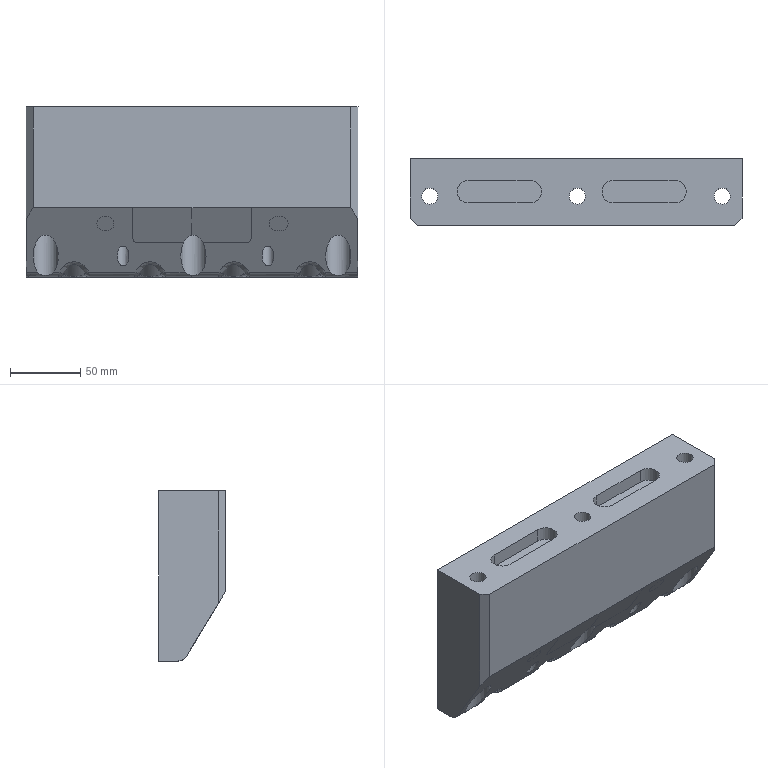Part | NX | features solid 2 | 1 solid | 65 faces | box 236 x 47.451 x 121.13 mm | volume 1087057 mm3 | spline 22 | cylinder 22 | plane 19 | cone 2 | commonest cylinder face diameters 15 x6 16 x4 21 x4 11.507 x3 18.008 x3 8.506 x2